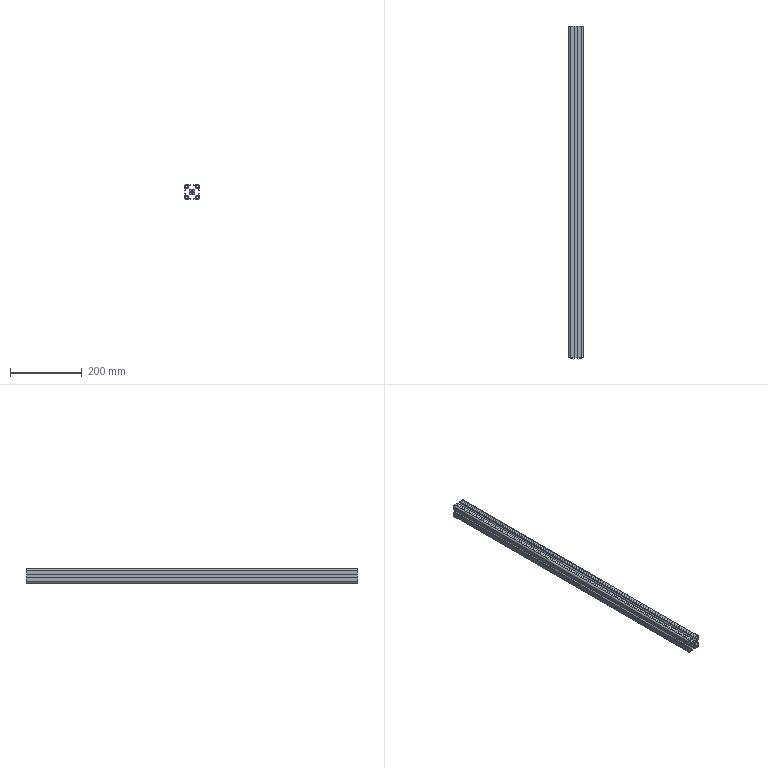Part | 1 solid | 104 faces | box 40 x 926 x 40 mm | volume 533881 mm3 | plane 94 | cylinder 10 | commonest cylinder face diameters 5 x4 9 x4 6.8 x2